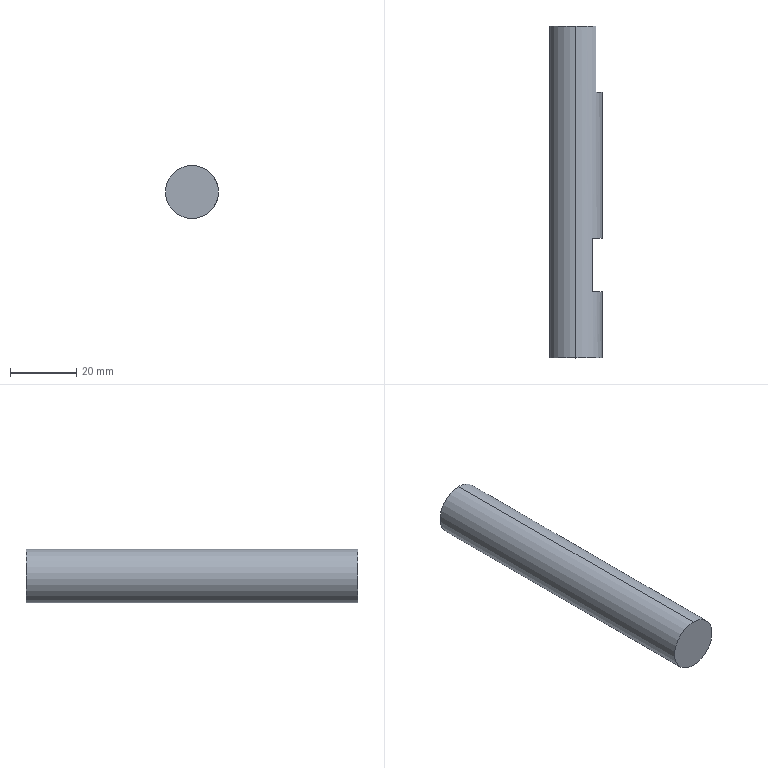Part | SolidWorks | features Extrusion 1, ICE 1 | 1 solid | 9 faces | box 16 x 100 x 16 mm | volume 19399 mm3 | plane 7 | cylinder 2 | commonest cylinder face diameters 16 x2
STEP:
#1=CARTESIAN_POINT('',(5.,36.,-6.245));
#2=VERTEX_POINT('',#1);
#3=CARTESIAN_POINT('',(5.,20.,-6.245));
#4=VERTEX_POINT('',#3);
#5=CARTESIAN_POINT('',(5.,100.,-6.245));
#6=DIRECTION('',(0.,-1.,0.));
#7=VECTOR('',#6,1000.);
#8=LINE('',#5,#7);
#9=EDGE_CURVE('',#2,#4,#8,.T.);
#10=ORIENTED_EDGE('',*,*,#9,.T.);
#11=CARTESIAN_POINT('',(5.,20.,6.245));
#12=VERTEX_POINT('',#11);
#13=CARTESIAN_POINT('',(0.,20.,0.));
#14=DIRECTION('',(0.,-1.,0.));
#15=DIRECTION('',(0.,0.,-1.));
#16=AXIS2_PLACEMENT_3D('',#13,#14,#15);
#17=CIRCLE('',#16,8.);
#18=EDGE_CURVE('',#4,#12,#17,.T.);
#19=ORIENTED_EDGE('',*,*,#18,.T.);
#20=CARTESIAN_POINT('',(5.,36.,6.245));
#21=VERTEX_POINT('',#20);
#22=CARTESIAN_POINT('',(5.,100.,6.245));
#23=DIRECTION('',(0.,1.,0.));
#24=VECTOR('',#23,1000.);
#25=LINE('',#22,#24);
#26=EDGE_CURVE('',#12,#21,#25,.T.);
#27=ORIENTED_EDGE('',*,*,#26,.T.);
#28=CARTESIAN_POINT('',(0.,36.,0.));
#29=DIRECTION('',(0.,1.,0.));
#30=DIRECTION('',(0.,0.,1.));
#31=AXIS2_PLACEMENT_3D('',#28,#29,#30);
#32=CIRCLE('',#31,8.);
#33=EDGE_CURVE('',#21,#2,#32,.T.);
#34=ORIENTED_EDGE('',*,*,#33,.T.);
#35=EDGE_LOOP('',(#10,#19,#27,#34));
#36=FACE_BOUND('',#35,.T.);
#37=CARTESIAN_POINT('',(0.,100.,8.));
#38=VERTEX_POINT('',#37);
#39=CARTESIAN_POINT('',(6.,100.,5.292));
#40=VERTEX_POINT('',#39);
#41=CARTESIAN_POINT('',(0.,100.,0.));
#42=DIRECTION('',(0.,1.,0.));
#43=DIRECTION('',(0.,0.,1.));
#44=AXIS2_PLACEMENT_3D('',#41,#42,#43);
#45=CIRCLE('',#44,8.);
#46=EDGE_CURVE('',#38,#40,#45,.T.);
#47=ORIENTED_EDGE('',*,*,#46,.F.);
#48=CARTESIAN_POINT('',(0.,0.,8.));
#49=VERTEX_POINT('',#48);
#50=CARTESIAN_POINT('',(0.,100.,8.));
#51=DIRECTION('',(0.,-1.,0.));
#52=VECTOR('',#51,1000.);
#53=LINE('',#50,#52);
#54=EDGE_CURVE('',#38,#49,#53,.T.);
#55=ORIENTED_EDGE('',*,*,#54,.T.);
#56=CARTESIAN_POINT('',(0.,0.,-8.));
#57=VERTEX_POINT('',#56);
#58=CARTESIAN_POINT('',(0.,0.,0.));
#59=DIRECTION('',(0.,1.,0.));
#60=DIRECTION('',(0.,0.,1.));
#61=AXIS2_PLACEMENT_3D('',#58,#59,#60);
#62=CIRCLE('',#61,8.);
#63=EDGE_CURVE('',#49,#57,#62,.T.);
#64=ORIENTED_EDGE('',*,*,#63,.T.);
#65=CARTESIAN_POINT('',(0.,100.,-8.));
#66=VERTEX_POINT('',#65);
#67=CARTESIAN_POINT('',(0.,100.,-8.));
#68=DIRECTION('',(0.,-1.,0.));
#69=VECTOR('',#68,1000.);
#70=LINE('',#67,#69);
#71=EDGE_CURVE('',#66,#57,#70,.T.);
#72=ORIENTED_EDGE('',*,*,#71,.F.);
#73=CARTESIAN_POINT('',(6.,100.,-5.292));
#74=VERTEX_POINT('',#73);
#75=CARTESIAN_POINT('',(0.,100.,0.));
#76=DIRECTION('',(0.,1.,0.));
#77=DIRECTION('',(0.,0.,1.));
#78=AXIS2_PLACEMENT_3D('',#75,#76,#77);
#79=CIRCLE('',#78,8.);
#80=EDGE_CURVE('',#74,#66,#79,.T.);
#81=ORIENTED_EDGE('',*,*,#80,.F.);
#82=CARTESIAN_POINT('',(6.,80.,-5.292));
#83=VERTEX_POINT('',#82);
#84=CARTESIAN_POINT('',(6.,100.,-5.292));
#85=DIRECTION('',(0.,-1.,0.));
#86=VECTOR('',#85,1000.);
#87=LINE('',#84,#86);
#88=EDGE_CURVE('',#74,#83,#87,.T.);
#89=ORIENTED_EDGE('',*,*,#88,.T.);
#90=CARTESIAN_POINT('',(6.,80.,5.292));
#91=VERTEX_POINT('',#90);
#92=CARTESIAN_POINT('',(0.,80.,0.));
#93=DIRECTION('',(0.,-1.,0.));
#94=DIRECTION('',(0.,0.,-1.));
#95=AXIS2_PLACEMENT_3D('',#92,#93,#94);
#96=CIRCLE('',#95,8.);
#97=EDGE_CURVE('',#83,#91,#96,.T.);
#98=ORIENTED_EDGE('',*,*,#97,.T.);
#99=CARTESIAN_POINT('',(6.,100.,5.292));
#100=DIRECTION('',(0.,1.,0.));
#101=VECTOR('',#100,1000.);
#102=LINE('',#99,#101);
#103=EDGE_CURVE('',#91,#40,#102,.T.);
#104=ORIENTED_EDGE('',*,*,#103,.T.);
#105=EDGE_LOOP('',(#47,#55,#64,#72,#81,#89,#98,#104));
#106=FACE_OUTER_BOUND('',#105,.T.);
#107=CARTESIAN_POINT('',(0.,100.,0.));
#108=DIRECTION('',(0.,-1.,0.));
#109=DIRECTION('',(0.,0.,-1.));
#110=AXIS2_PLACEMENT_3D('',#107,#108,#109);
#111=CYLINDRICAL_SURFACE('',#110,8.);
#112=ADVANCED_FACE('',(#36,#106),#111,.T.);
#113=ORIENTED_EDGE('',*,*,#54,.F.);
#114=CARTESIAN_POINT('',(0.,100.,0.));
#115=DIRECTION('',(0.,1.,0.));
#116=DIRECTION('',(0.,0.,1.));
#117=AXIS2_PLACEMENT_3D('',#114,#115,#116);
#118=CIRCLE('',#117,8.);
#119=EDGE_CURVE('',#66,#38,#118,.T.);
#120=ORIENTED_EDGE('',*,*,#119,.F.);
#121=ORIENTED_EDGE('',*,*,#71,.T.);
#122=CARTESIAN_POINT('',(0.,0.,0.));
#123=DIRECTION('',(0.,1.,0.));
#124=DIRECTION('',(0.,0.,1.));
#125=AXIS2_PLACEMENT_3D('',#122,#123,#124);
#126=CIRCLE('',#125,8.);
#127=EDGE_CURVE('',#57,#49,#126,.T.);
#128=ORIENTED_EDGE('',*,*,#127,.T.);
#129=EDGE_LOOP('',(#113,#120,#121,#128));
#130=FACE_OUTER_BOUND('',#129,.T.);
#131=CARTESIAN_POINT('',(0.,100.,0.));
#132=DIRECTION('',(0.,-1.,0.));
#133=DIRECTION('',(0.,0.,-1.));
#134=AXIS2_PLACEMENT_3D('',#131,#132,#133);
#135=CYLINDRICAL_SURFACE('',#134,8.);
#136=ADVANCED_FACE('',(#130),#135,.T.);
#137=CARTESIAN_POINT('',(6.,100.,0.));
#138=DIRECTION('',(0.,0.,1.));
#139=VECTOR('',#138,1000.);
#140=LINE('',#137,#139);
#141=EDGE_CURVE('',#74,#40,#140,.T.);
#142=ORIENTED_EDGE('',*,*,#141,.F.);
#143=ORIENTED_EDGE('',*,*,#80,.T.);
#144=ORIENTED_EDGE('',*,*,#119,.T.);
#145=ORIENTED_EDGE('',*,*,#46,.T.);
#146=EDGE_LOOP('',(#142,#143,#144,#145));
#147=FACE_OUTER_BOUND('',#146,.T.);
#148=CARTESIAN_POINT('',(0.,100.,0.));
#149=DIRECTION('',(0.,1.,0.));
#150=DIRECTION('',(0.,0.,1.));
#151=AXIS2_PLACEMENT_3D('',#148,#149,#150);
#152=PLANE('',#151);
#153=ADVANCED_FACE('',(#147),#152,.T.);
#154=ORIENTED_EDGE('',*,*,#127,.F.);
#155=ORIENTED_EDGE('',*,*,#63,.F.);
#156=EDGE_LOOP('',(#154,#155));
#157=FACE_OUTER_BOUND('',#156,.T.);
#158=CARTESIAN_POINT('',(0.,0.,0.));
#159=DIRECTION('',(0.,1.,0.));
#160=DIRECTION('',(0.,0.,1.));
#161=AXIS2_PLACEMENT_3D('',#158,#159,#160);
#162=PLANE('',#161);
#163=ADVANCED_FACE('',(#157),#162,.F.);
#164=CARTESIAN_POINT('',(6.,80.,-8.));
#165=DIRECTION('',(0.,0.,1.));
#166=VECTOR('',#165,1000.);
#167=LINE('',#164,#166);
#168=EDGE_CURVE('',#83,#91,#167,.T.);
#169=ORIENTED_EDGE('',*,*,#168,.T.);
#170=ORIENTED_EDGE('',*,*,#97,.F.);
#171=EDGE_LOOP('',(#169,#170));
#172=FACE_OUTER_BOUND('',#171,.T.);
#173=CARTESIAN_POINT('',(8.,80.,-8.));
#174=DIRECTION('',(0.,-1.,0.));
#175=DIRECTION('',(0.,0.,-1.));
#176=AXIS2_PLACEMENT_3D('',#173,#174,#175);
#177=PLANE('',#176);
#178=ADVANCED_FACE('',(#172),#177,.F.);
#179=ORIENTED_EDGE('',*,*,#141,.T.);
#180=ORIENTED_EDGE('',*,*,#103,.F.);
#181=ORIENTED_EDGE('',*,*,#168,.F.);
#182=ORIENTED_EDGE('',*,*,#88,.F.);
#183=EDGE_LOOP('',(#179,#180,#181,#182));
#184=FACE_OUTER_BOUND('',#183,.T.);
#185=CARTESIAN_POINT('',(6.,80.,-8.));
#186=DIRECTION('',(-1.,0.,0.));
#187=DIRECTION('',(0.,0.,1.));
#188=AXIS2_PLACEMENT_3D('',#185,#186,#187);
#189=PLANE('',#188);
#190=ADVANCED_FACE('',(#184),#189,.F.);
#191=CARTESIAN_POINT('',(5.,20.,-8.));
#192=DIRECTION('',(0.,0.,1.));
#193=VECTOR('',#192,1000.);
#194=LINE('',#191,#193);
#195=EDGE_CURVE('',#4,#12,#194,.T.);
#196=ORIENTED_EDGE('',*,*,#195,.T.);
#197=ORIENTED_EDGE('',*,*,#18,.F.);
#198=EDGE_LOOP('',(#196,#197));
#199=FACE_OUTER_BOUND('',#198,.T.);
#200=CARTESIAN_POINT('',(5.,20.,-8.));
#201=DIRECTION('',(0.,-1.,0.));
#202=DIRECTION('',(0.,0.,-1.));
#203=AXIS2_PLACEMENT_3D('',#200,#201,#202);
#204=PLANE('',#203);
#205=ADVANCED_FACE('',(#199),#204,.F.);
#206=CARTESIAN_POINT('',(5.,36.,-8.));
#207=DIRECTION('',(0.,0.,1.));
#208=VECTOR('',#207,1000.);
#209=LINE('',#206,#208);
#210=EDGE_CURVE('',#2,#21,#209,.T.);
#211=ORIENTED_EDGE('',*,*,#210,.T.);
#212=ORIENTED_EDGE('',*,*,#26,.F.);
#213=ORIENTED_EDGE('',*,*,#195,.F.);
#214=ORIENTED_EDGE('',*,*,#9,.F.);
#215=EDGE_LOOP('',(#211,#212,#213,#214));
#216=FACE_OUTER_BOUND('',#215,.T.);
#217=CARTESIAN_POINT('',(5.,36.,-8.));
#218=DIRECTION('',(-1.,0.,0.));
#219=DIRECTION('',(0.,-1.,0.));
#220=AXIS2_PLACEMENT_3D('',#217,#218,#219);
#221=PLANE('',#220);
#222=ADVANCED_FACE('',(#216),#221,.F.);
#223=ORIENTED_EDGE('',*,*,#210,.F.);
#224=ORIENTED_EDGE('',*,*,#33,.F.);
#225=EDGE_LOOP('',(#223,#224));
#226=FACE_OUTER_BOUND('',#225,.T.);
#227=CARTESIAN_POINT('',(5.,36.,-8.));
#228=DIRECTION('',(0.,1.,0.));
#229=DIRECTION('',(0.,0.,1.));
#230=AXIS2_PLACEMENT_3D('',#227,#228,#229);
#231=PLANE('',#230);
#232=ADVANCED_FACE('',(#226),#231,.F.);
#233=CLOSED_SHELL('',(#112,#136,#153,#163,#178,#190,#205,#222,#232));
#234=MANIFOLD_SOLID_BREP('',#233);
#235=CARTESIAN_POINT('',(0.,0.,0.));
#236=DIRECTION('',(0.,0.,1.));
#237=DIRECTION('',(1.,0.,0.));
#238=AXIS2_PLACEMENT_3D('',#235,#236,#237);
#239=(LENGTH_UNIT()NAMED_UNIT(*)SI_UNIT(.MILLI.,.METRE.));
#240=UNCERTAINTY_MEASURE_WITH_UNIT(LENGTH_MEASURE(0.00001),#239,'','');
#241=(NAMED_UNIT(*)PLANE_ANGLE_UNIT()SI_UNIT($,.RADIAN.));
#242=(NAMED_UNIT(*)SI_UNIT($,.STERADIAN.)SOLID_ANGLE_UNIT());
#243=(GEOMETRIC_REPRESENTATION_CONTEXT(3)GLOBAL_UNCERTAINTY_ASSIGNED_CONTEXT((#240))GLOBAL_UNIT_ASSIGNED_CONTEXT((#239,#241,#242))REPRESENTATION_CONTEXT('',''));
#244=ADVANCED_BREP_SHAPE_REPRESENTATION('',(#234,#238),#243);